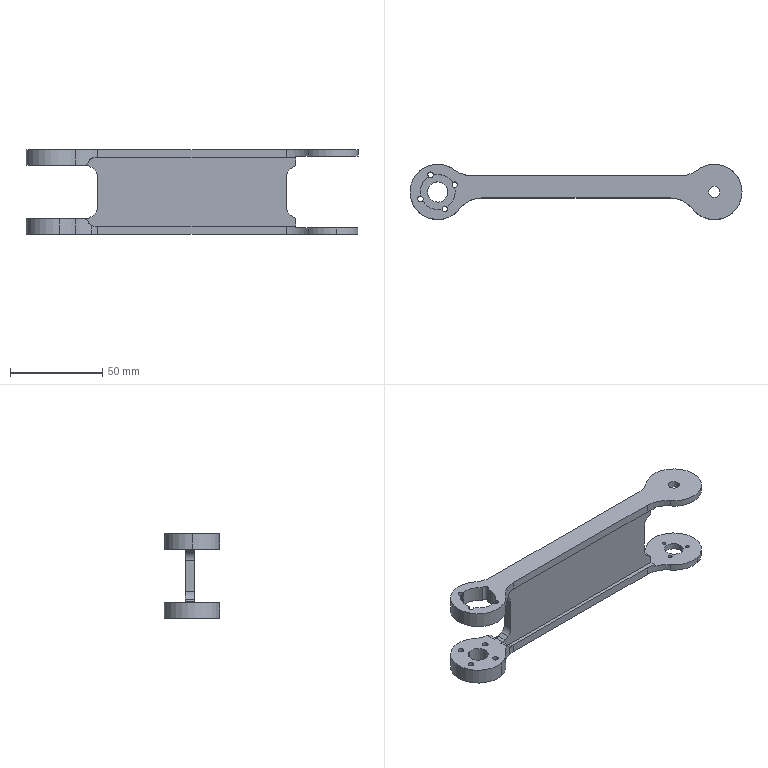Part | NX | features BREP 1 | 1 solid | 111 faces | box 180 x 30 x 46 mm | volume 37069 mm3 | cylinder 76 | plane 35 | commonest cylinder face diameters 30 x18 3 x17 10 x14 6 x12 2 x6 19 x5